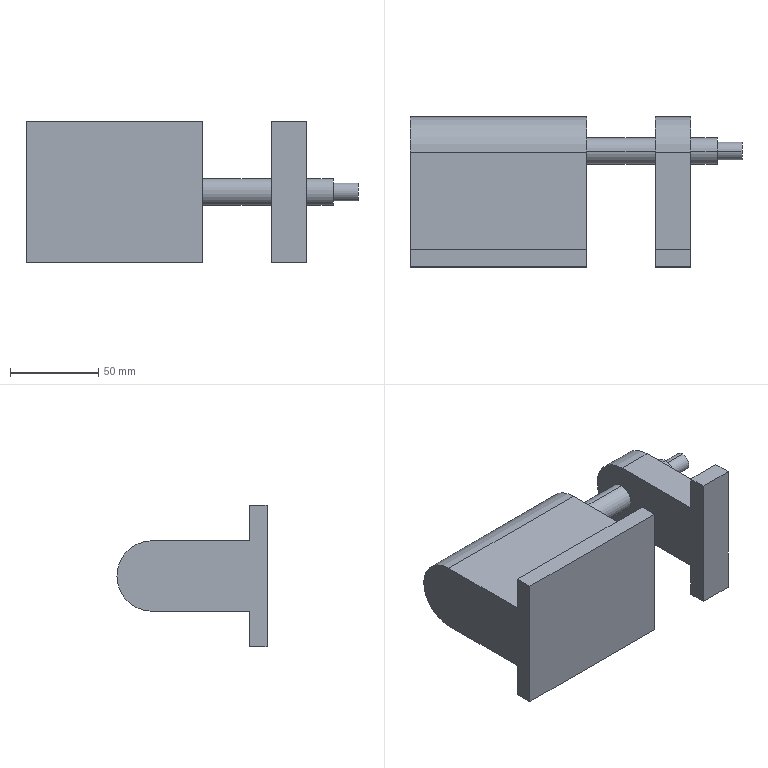Part | SolidWorks | features BaseBody 1 | 1 solid | 30 faces | box 188 x 85 x 80 mm | volume 446040 mm3 | plane 20 | cylinder 10 | commonest cylinder face diameters 15 x4 40 x4 10 x2
STEP:
#1=CARTESIAN_POINT('',(172.311,72.768,44.5));
#2=VERTEX_POINT('',#1);
#3=CARTESIAN_POINT('',(172.311,72.768,54.5));
#4=VERTEX_POINT('',#3);
#5=CARTESIAN_POINT('',(172.311,72.768,49.5));
#6=DIRECTION('',(1.,0.,0.));
#7=DIRECTION('',(0.,0.,-1.));
#8=AXIS2_PLACEMENT_3D('',#5,#6,#7);
#9=CIRCLE('',#8,5.);
#10=EDGE_CURVE('',#2,#4,#9,.T.);
#11=ORIENTED_EDGE('',*,*,#10,.F.);
#12=CARTESIAN_POINT('',(158.311,72.768,44.5));
#13=VERTEX_POINT('',#12);
#14=CARTESIAN_POINT('',(172.311,72.768,44.5));
#15=DIRECTION('',(-1.,0.,0.));
#16=VECTOR('',#15,1000.);
#17=LINE('',#14,#16);
#18=EDGE_CURVE('',#2,#13,#17,.T.);
#19=ORIENTED_EDGE('',*,*,#18,.T.);
#20=CARTESIAN_POINT('',(158.311,72.768,54.5));
#21=VERTEX_POINT('',#20);
#22=CARTESIAN_POINT('',(158.311,72.768,49.5));
#23=DIRECTION('',(1.,0.,0.));
#24=DIRECTION('',(0.,0.,-1.));
#25=AXIS2_PLACEMENT_3D('',#22,#23,#24);
#26=CIRCLE('',#25,5.);
#27=EDGE_CURVE('',#13,#21,#26,.T.);
#28=ORIENTED_EDGE('',*,*,#27,.T.);
#29=CARTESIAN_POINT('',(172.311,72.768,54.5));
#30=DIRECTION('',(-1.,0.,0.));
#31=VECTOR('',#30,1000.);
#32=LINE('',#29,#31);
#33=EDGE_CURVE('',#4,#21,#32,.T.);
#34=ORIENTED_EDGE('',*,*,#33,.F.);
#35=EDGE_LOOP('',(#11,#19,#28,#34));
#36=FACE_OUTER_BOUND('',#35,.T.);
#37=CARTESIAN_POINT('',(172.311,72.768,49.5));
#38=DIRECTION('',(-1.,0.,0.));
#39=DIRECTION('',(0.,0.,1.));
#40=AXIS2_PLACEMENT_3D('',#37,#38,#39);
#41=CYLINDRICAL_SURFACE('',#40,5.);
#42=ADVANCED_FACE('',(#36),#41,.T.);
#43=CARTESIAN_POINT('',(158.311,72.768,42.));
#44=VERTEX_POINT('',#43);
#45=CARTESIAN_POINT('',(158.311,72.768,57.));
#46=VERTEX_POINT('',#45);
#47=CARTESIAN_POINT('',(158.311,72.768,49.5));
#48=DIRECTION('',(1.,0.,0.));
#49=DIRECTION('',(0.,0.,-1.));
#50=AXIS2_PLACEMENT_3D('',#47,#48,#49);
#51=CIRCLE('',#50,7.5);
#52=EDGE_CURVE('',#44,#46,#51,.T.);
#53=ORIENTED_EDGE('',*,*,#52,.F.);
#54=CARTESIAN_POINT('',(143.218,72.768,42.));
#55=VERTEX_POINT('',#54);
#56=CARTESIAN_POINT('',(158.311,72.768,42.));
#57=DIRECTION('',(-1.,0.,0.));
#58=VECTOR('',#57,1000.);
#59=LINE('',#56,#58);
#60=EDGE_CURVE('',#44,#55,#59,.T.);
#61=ORIENTED_EDGE('',*,*,#60,.T.);
#62=CARTESIAN_POINT('',(143.218,72.768,57.));
#63=VERTEX_POINT('',#62);
#64=CARTESIAN_POINT('',(143.218,72.768,49.5));
#65=DIRECTION('',(1.,0.,0.));
#66=DIRECTION('',(0.,0.,-1.));
#67=AXIS2_PLACEMENT_3D('',#64,#65,#66);
#68=CIRCLE('',#67,7.5);
#69=EDGE_CURVE('',#55,#63,#68,.T.);
#70=ORIENTED_EDGE('',*,*,#69,.T.);
#71=CARTESIAN_POINT('',(158.311,72.768,57.));
#72=DIRECTION('',(-1.,0.,0.));
#73=VECTOR('',#72,1000.);
#74=LINE('',#71,#73);
#75=EDGE_CURVE('',#46,#63,#74,.T.);
#76=ORIENTED_EDGE('',*,*,#75,.F.);
#77=EDGE_LOOP('',(#53,#61,#70,#76));
#78=FACE_OUTER_BOUND('',#77,.T.);
#79=CARTESIAN_POINT('',(158.311,72.768,49.5));
#80=DIRECTION('',(-1.,0.,0.));
#81=DIRECTION('',(0.,0.,1.));
#82=AXIS2_PLACEMENT_3D('',#79,#80,#81);
#83=CYLINDRICAL_SURFACE('',#82,7.5);
#84=ADVANCED_FACE('',(#78),#83,.T.);
#85=CARTESIAN_POINT('',(123.218,72.768,57.));
#86=VERTEX_POINT('',#85);
#87=CARTESIAN_POINT('',(123.218,72.768,42.));
#88=VERTEX_POINT('',#87);
#89=CARTESIAN_POINT('',(123.218,72.768,49.5));
#90=DIRECTION('',(-1.,0.,0.));
#91=DIRECTION('',(0.,0.,-1.));
#92=AXIS2_PLACEMENT_3D('',#89,#90,#91);
#93=CIRCLE('',#92,7.5);
#94=EDGE_CURVE('',#86,#88,#93,.T.);
#95=ORIENTED_EDGE('',*,*,#94,.T.);
#96=CARTESIAN_POINT('',(84.311,72.768,42.));
#97=VERTEX_POINT('',#96);
#98=CARTESIAN_POINT('',(158.311,72.768,42.));
#99=DIRECTION('',(-1.,0.,0.));
#100=VECTOR('',#99,1000.);
#101=LINE('',#98,#100);
#102=EDGE_CURVE('',#88,#97,#101,.T.);
#103=ORIENTED_EDGE('',*,*,#102,.T.);
#104=CARTESIAN_POINT('',(84.311,72.768,57.));
#105=VERTEX_POINT('',#104);
#106=CARTESIAN_POINT('',(84.311,72.768,49.5));
#107=DIRECTION('',(1.,0.,0.));
#108=DIRECTION('',(0.,0.,1.));
#109=AXIS2_PLACEMENT_3D('',#106,#107,#108);
#110=CIRCLE('',#109,7.5);
#111=EDGE_CURVE('',#97,#105,#110,.T.);
#112=ORIENTED_EDGE('',*,*,#111,.T.);
#113=CARTESIAN_POINT('',(158.311,72.768,57.));
#114=DIRECTION('',(-1.,0.,0.));
#115=VECTOR('',#114,1000.);
#116=LINE('',#113,#115);
#117=EDGE_CURVE('',#86,#105,#116,.T.);
#118=ORIENTED_EDGE('',*,*,#117,.F.);
#119=EDGE_LOOP('',(#95,#103,#112,#118));
#120=FACE_OUTER_BOUND('',#119,.T.);
#121=CARTESIAN_POINT('',(158.311,72.768,49.5));
#122=DIRECTION('',(-1.,0.,0.));
#123=DIRECTION('',(0.,0.,1.));
#124=AXIS2_PLACEMENT_3D('',#121,#122,#123);
#125=CYLINDRICAL_SURFACE('',#124,7.5);
#126=ADVANCED_FACE('',(#120),#125,.T.);
#127=CARTESIAN_POINT('',(158.311,72.768,49.5));
#128=DIRECTION('',(1.,0.,0.));
#129=DIRECTION('',(0.,0.,-1.));
#130=AXIS2_PLACEMENT_3D('',#127,#128,#129);
#131=CIRCLE('',#130,7.5);
#132=EDGE_CURVE('',#46,#44,#131,.T.);
#133=ORIENTED_EDGE('',*,*,#132,.T.);
#134=ORIENTED_EDGE('',*,*,#52,.T.);
#135=EDGE_LOOP('',(#133,#134));
#136=FACE_OUTER_BOUND('',#135,.T.);
#137=CARTESIAN_POINT('',(158.311,72.768,49.5));
#138=DIRECTION('',(1.,0.,0.));
#139=DIRECTION('',(0.,0.,-1.));
#140=AXIS2_PLACEMENT_3D('',#137,#138,#139);
#141=CIRCLE('',#140,5.);
#142=EDGE_CURVE('',#21,#13,#141,.T.);
#143=ORIENTED_EDGE('',*,*,#142,.F.);
#144=ORIENTED_EDGE('',*,*,#27,.F.);
#145=EDGE_LOOP('',(#143,#144));
#146=FACE_BOUND('',#145,.T.);
#147=CARTESIAN_POINT('',(158.311,72.768,49.5));
#148=DIRECTION('',(1.,0.,0.));
#149=DIRECTION('',(0.,0.,-1.));
#150=AXIS2_PLACEMENT_3D('',#147,#148,#149);
#151=PLANE('',#150);
#152=ADVANCED_FACE('',(#136,#146),#151,.T.);
#153=CARTESIAN_POINT('',(84.311,72.138,29.5));
#154=VERTEX_POINT('',#153);
#155=CARTESIAN_POINT('',(84.311,17.138,29.5));
#156=VERTEX_POINT('',#155);
#157=CARTESIAN_POINT('',(84.311,92.138,29.5));
#158=DIRECTION('',(0.,-1.,0.));
#159=VECTOR('',#158,1000.);
#160=LINE('',#157,#159);
#161=EDGE_CURVE('',#154,#156,#160,.T.);
#162=ORIENTED_EDGE('',*,*,#161,.F.);
#163=CARTESIAN_POINT('',(84.311,92.138,49.5));
#164=VERTEX_POINT('',#163);
#165=CARTESIAN_POINT('',(84.311,72.138,49.5));
#166=DIRECTION('',(1.,0.,0.));
#167=DIRECTION('',(0.,0.,1.));
#168=AXIS2_PLACEMENT_3D('',#165,#166,#167);
#169=CIRCLE('',#168,20.);
#170=EDGE_CURVE('',#154,#164,#169,.T.);
#171=ORIENTED_EDGE('',*,*,#170,.T.);
#172=CARTESIAN_POINT('',(84.311,72.138,69.5));
#173=VERTEX_POINT('',#172);
#174=CARTESIAN_POINT('',(84.311,72.138,49.5));
#175=DIRECTION('',(1.,0.,0.));
#176=DIRECTION('',(0.,0.,1.));
#177=AXIS2_PLACEMENT_3D('',#174,#175,#176);
#178=CIRCLE('',#177,20.);
#179=EDGE_CURVE('',#164,#173,#178,.T.);
#180=ORIENTED_EDGE('',*,*,#179,.T.);
#181=CARTESIAN_POINT('',(84.311,17.138,69.5));
#182=VERTEX_POINT('',#181);
#183=CARTESIAN_POINT('',(84.311,92.138,69.5));
#184=DIRECTION('',(0.,-1.,0.));
#185=VECTOR('',#184,1000.);
#186=LINE('',#183,#185);
#187=EDGE_CURVE('',#173,#182,#186,.T.);
#188=ORIENTED_EDGE('',*,*,#187,.T.);
#189=CARTESIAN_POINT('',(84.311,17.138,89.5));
#190=VERTEX_POINT('',#189);
#191=CARTESIAN_POINT('',(84.311,17.138,89.5));
#192=DIRECTION('',(0.,0.,-1.));
#193=VECTOR('',#192,1000.);
#194=LINE('',#191,#193);
#195=EDGE_CURVE('',#190,#182,#194,.T.);
#196=ORIENTED_EDGE('',*,*,#195,.F.);
#197=CARTESIAN_POINT('',(84.311,7.138,89.5));
#198=VERTEX_POINT('',#197);
#199=CARTESIAN_POINT('',(84.311,17.138,89.5));
#200=DIRECTION('',(0.,-1.,0.));
#201=VECTOR('',#200,1000.);
#202=LINE('',#199,#201);
#203=EDGE_CURVE('',#190,#198,#202,.T.);
#204=ORIENTED_EDGE('',*,*,#203,.T.);
#205=CARTESIAN_POINT('',(84.311,7.138,9.5));
#206=VERTEX_POINT('',#205);
#207=CARTESIAN_POINT('',(84.311,7.138,89.5));
#208=DIRECTION('',(0.,0.,-1.));
#209=VECTOR('',#208,1000.);
#210=LINE('',#207,#209);
#211=EDGE_CURVE('',#198,#206,#210,.T.);
#212=ORIENTED_EDGE('',*,*,#211,.T.);
#213=CARTESIAN_POINT('',(84.311,17.138,9.5));
#214=VERTEX_POINT('',#213);
#215=CARTESIAN_POINT('',(84.311,17.138,9.5));
#216=DIRECTION('',(0.,-1.,0.));
#217=VECTOR('',#216,1000.);
#218=LINE('',#215,#217);
#219=EDGE_CURVE('',#214,#206,#218,.T.);
#220=ORIENTED_EDGE('',*,*,#219,.F.);
#221=CARTESIAN_POINT('',(84.311,17.138,89.5));
#222=DIRECTION('',(0.,0.,-1.));
#223=VECTOR('',#222,1000.);
#224=LINE('',#221,#223);
#225=EDGE_CURVE('',#156,#214,#224,.T.);
#226=ORIENTED_EDGE('',*,*,#225,.F.);
#227=EDGE_LOOP('',(#162,#171,#180,#188,#196,#204,#212,#220,#226));
#228=FACE_OUTER_BOUND('',#227,.T.);
#229=CARTESIAN_POINT('',(84.311,72.768,49.5));
#230=DIRECTION('',(1.,0.,0.));
#231=DIRECTION('',(0.,0.,1.));
#232=AXIS2_PLACEMENT_3D('',#229,#230,#231);
#233=CIRCLE('',#232,7.5);
#234=EDGE_CURVE('',#105,#97,#233,.T.);
#235=ORIENTED_EDGE('',*,*,#234,.F.);
#236=ORIENTED_EDGE('',*,*,#111,.F.);
#237=EDGE_LOOP('',(#235,#236));
#238=FACE_BOUND('',#237,.T.);
#239=CARTESIAN_POINT('',(84.311,17.138,89.5));
#240=DIRECTION('',(-1.,0.,0.));
#241=DIRECTION('',(0.,0.,1.));
#242=AXIS2_PLACEMENT_3D('',#239,#240,#241);
#243=PLANE('',#242);
#244=ADVANCED_FACE('',(#228,#238),#243,.F.);
#245=CARTESIAN_POINT('',(-15.689,17.138,69.5));
#246=VERTEX_POINT('',#245);
#247=CARTESIAN_POINT('',(84.311,17.138,69.5));
#248=DIRECTION('',(1.,0.,0.));
#249=VECTOR('',#248,1000.);
#250=LINE('',#247,#249);
#251=EDGE_CURVE('',#246,#182,#250,.T.);
#252=ORIENTED_EDGE('',*,*,#251,.F.);
#253=CARTESIAN_POINT('',(-15.689,17.138,89.5));
#254=VERTEX_POINT('',#253);
#255=CARTESIAN_POINT('',(-15.689,17.138,9.5));
#256=DIRECTION('',(0.,0.,1.));
#257=VECTOR('',#256,1000.);
#258=LINE('',#255,#257);
#259=EDGE_CURVE('',#246,#254,#258,.T.);
#260=ORIENTED_EDGE('',*,*,#259,.T.);
#261=CARTESIAN_POINT('',(-15.689,17.138,89.5));
#262=DIRECTION('',(1.,0.,0.));
#263=VECTOR('',#262,1000.);
#264=LINE('',#261,#263);
#265=EDGE_CURVE('',#254,#190,#264,.T.);
#266=ORIENTED_EDGE('',*,*,#265,.T.);
#267=ORIENTED_EDGE('',*,*,#195,.T.);
#268=EDGE_LOOP('',(#252,#260,#266,#267));
#269=FACE_OUTER_BOUND('',#268,.T.);
#270=CARTESIAN_POINT('',(-546.782,17.138,0.));
#271=DIRECTION('',(0.,1.,0.));
#272=DIRECTION('',(0.,0.,1.));
#273=AXIS2_PLACEMENT_3D('',#270,#271,#272);
#274=PLANE('',#273);
#275=ADVANCED_FACE('',(#269),#274,.T.);
#276=CARTESIAN_POINT('',(123.218,17.138,69.5));
#277=VERTEX_POINT('',#276);
#278=CARTESIAN_POINT('',(143.218,17.138,69.5));
#279=VERTEX_POINT('',#278);
#280=CARTESIAN_POINT('',(123.218,17.138,69.5));
#281=DIRECTION('',(1.,0.,0.));
#282=VECTOR('',#281,1000.);
#283=LINE('',#280,#282);
#284=EDGE_CURVE('',#277,#279,#283,.T.);
#285=ORIENTED_EDGE('',*,*,#284,.F.);
#286=CARTESIAN_POINT('',(123.218,17.138,89.5));
#287=VERTEX_POINT('',#286);
#288=CARTESIAN_POINT('',(123.218,17.138,15.727));
#289=DIRECTION('',(0.,0.,1.));
#290=VECTOR('',#289,1000.);
#291=LINE('',#288,#290);
#292=EDGE_CURVE('',#277,#287,#291,.T.);
#293=ORIENTED_EDGE('',*,*,#292,.T.);
#294=CARTESIAN_POINT('',(143.218,17.138,89.5));
#295=VERTEX_POINT('',#294);
#296=CARTESIAN_POINT('',(123.218,17.138,89.5));
#297=DIRECTION('',(1.,0.,0.));
#298=VECTOR('',#297,1000.);
#299=LINE('',#296,#298);
#300=EDGE_CURVE('',#287,#295,#299,.T.);
#301=ORIENTED_EDGE('',*,*,#300,.T.);
#302=CARTESIAN_POINT('',(143.218,17.138,15.727));
#303=DIRECTION('',(0.,0.,-1.));
#304=VECTOR('',#303,1000.);
#305=LINE('',#302,#304);
#306=EDGE_CURVE('',#295,#279,#305,.T.);
#307=ORIENTED_EDGE('',*,*,#306,.T.);
#308=EDGE_LOOP('',(#285,#293,#301,#307));
#309=FACE_OUTER_BOUND('',#308,.T.);
#310=CARTESIAN_POINT('',(-546.782,17.138,0.));
#311=DIRECTION('',(0.,-1.,0.));
#312=DIRECTION('',(0.,0.,-1.));
#313=AXIS2_PLACEMENT_3D('',#310,#311,#312);
#314=PLANE('',#313);
#315=ADVANCED_FACE('',(#309),#314,.F.);
#316=CARTESIAN_POINT('',(143.218,17.138,29.5));
#317=VERTEX_POINT('',#316);
#318=CARTESIAN_POINT('',(123.218,17.138,29.5));
#319=VERTEX_POINT('',#318);
#320=CARTESIAN_POINT('',(123.218,17.138,29.5));
#321=DIRECTION('',(-1.,0.,0.));
#322=VECTOR('',#321,1000.);
#323=LINE('',#320,#322);
#324=EDGE_CURVE('',#317,#319,#323,.T.);
#325=ORIENTED_EDGE('',*,*,#324,.F.);
#326=CARTESIAN_POINT('',(143.218,17.138,9.5));
#327=VERTEX_POINT('',#326);
#328=CARTESIAN_POINT('',(143.218,17.138,15.727));
#329=DIRECTION('',(0.,0.,-1.));
#330=VECTOR('',#329,1000.);
#331=LINE('',#328,#330);
#332=EDGE_CURVE('',#317,#327,#331,.T.);
#333=ORIENTED_EDGE('',*,*,#332,.T.);
#334=CARTESIAN_POINT('',(123.218,17.138,9.5));
#335=VERTEX_POINT('',#334);
#336=CARTESIAN_POINT('',(123.218,17.138,9.5));
#337=DIRECTION('',(-1.,0.,0.));
#338=VECTOR('',#337,1000.);
#339=LINE('',#336,#338);
#340=EDGE_CURVE('',#327,#335,#339,.T.);
#341=ORIENTED_EDGE('',*,*,#340,.T.);
#342=CARTESIAN_POINT('',(123.218,17.138,15.727));
#343=DIRECTION('',(0.,0.,1.));
#344=VECTOR('',#343,1000.);
#345=LINE('',#342,#344);
#346=EDGE_CURVE('',#335,#319,#345,.T.);
#347=ORIENTED_EDGE('',*,*,#346,.T.);
#348=EDGE_LOOP('',(#325,#333,#341,#347));
#349=FACE_OUTER_BOUND('',#348,.T.);
#350=CARTESIAN_POINT('',(-546.782,17.138,0.));
#351=DIRECTION('',(0.,-1.,0.));
#352=DIRECTION('',(0.,0.,-1.));
#353=AXIS2_PLACEMENT_3D('',#350,#351,#352);
#354=PLANE('',#353);
#355=ADVANCED_FACE('',(#349),#354,.F.);
#356=CARTESIAN_POINT('',(143.218,7.138,9.5));
#357=VERTEX_POINT('',#356);
#358=CARTESIAN_POINT('',(123.218,7.138,9.5));
#359=VERTEX_POINT('',#358);
#360=CARTESIAN_POINT('',(123.218,7.138,9.5));
#361=DIRECTION('',(-1.,0.,0.));
#362=VECTOR('',#361,1000.);
#363=LINE('',#360,#362);
#364=EDGE_CURVE('',#357,#359,#363,.T.);
#365=ORIENTED_EDGE('',*,*,#364,.T.);
#366=CARTESIAN_POINT('',(123.218,17.138,9.5));
#367=DIRECTION('',(0.,-1.,0.));
#368=VECTOR('',#367,1000.);
#369=LINE('',#366,#368);
#370=EDGE_CURVE('',#335,#359,#369,.T.);
#371=ORIENTED_EDGE('',*,*,#370,.F.);
#372=ORIENTED_EDGE('',*,*,#340,.F.);
#373=CARTESIAN_POINT('',(143.218,17.138,9.5));
#374=DIRECTION('',(0.,-1.,0.));
#375=VECTOR('',#374,1000.);
#376=LINE('',#373,#375);
#377=EDGE_CURVE('',#327,#357,#376,.T.);
#378=ORIENTED_EDGE('',*,*,#377,.T.);
#379=EDGE_LOOP('',(#365,#371,#372,#378));
#380=FACE_OUTER_BOUND('',#379,.T.);
#381=CARTESIAN_POINT('',(123.218,17.138,9.5));
#382=DIRECTION('',(0.,0.,1.));
#383=DIRECTION('',(1.,0.,0.));
#384=AXIS2_PLACEMENT_3D('',#381,#382,#383);
#385=PLANE('',#384);
#386=ADVANCED_FACE('',(#380),#385,.F.);
#387=ORIENTED_EDGE('',*,*,#94,.F.);
#388=CARTESIAN_POINT('',(123.218,72.768,49.5));
#389=DIRECTION('',(-1.,0.,0.));
#390=DIRECTION('',(0.,0.,-1.));
#391=AXIS2_PLACEMENT_3D('',#388,#389,#390);
#392=CIRCLE('',#391,7.5);
#393=EDGE_CURVE('',#88,#86,#392,.T.);
#394=ORIENTED_EDGE('',*,*,#393,.F.);
#395=EDGE_LOOP('',(#387,#394));
#396=FACE_BOUND('',#395,.T.);
#397=CARTESIAN_POINT('',(123.218,72.138,69.5));
#398=VERTEX_POINT('',#397);
#399=CARTESIAN_POINT('',(123.218,92.138,49.5));
#400=VERTEX_POINT('',#399);
#401=CARTESIAN_POINT('',(123.218,72.138,49.5));
#402=DIRECTION('',(-1.,0.,0.));
#403=DIRECTION('',(0.,0.,-1.));
#404=AXIS2_PLACEMENT_3D('',#401,#402,#403);
#405=CIRCLE('',#404,20.);
#406=EDGE_CURVE('',#398,#400,#405,.T.);
#407=ORIENTED_EDGE('',*,*,#406,.T.);
#408=CARTESIAN_POINT('',(123.218,72.138,29.5));
#409=VERTEX_POINT('',#408);
#410=CARTESIAN_POINT('',(123.218,72.138,49.5));
#411=DIRECTION('',(-1.,0.,0.));
#412=DIRECTION('',(0.,0.,-1.));
#413=AXIS2_PLACEMENT_3D('',#410,#411,#412);
#414=CIRCLE('',#413,20.);
#415=EDGE_CURVE('',#400,#409,#414,.T.);
#416=ORIENTED_EDGE('',*,*,#415,.T.);
#417=CARTESIAN_POINT('',(123.218,92.138,29.5));
#418=DIRECTION('',(0.,-1.,0.));
#419=VECTOR('',#418,1000.);
#420=LINE('',#417,#419);
#421=EDGE_CURVE('',#409,#319,#420,.T.);
#422=ORIENTED_EDGE('',*,*,#421,.T.);
#423=ORIENTED_EDGE('',*,*,#346,.F.);
#424=ORIENTED_EDGE('',*,*,#370,.T.);
#425=CARTESIAN_POINT('',(123.218,7.138,89.5));
#426=VERTEX_POINT('',#425);
#427=CARTESIAN_POINT('',(123.218,7.138,15.727));
#428=DIRECTION('',(0.,0.,1.));
#429=VECTOR('',#428,1000.);
#430=LINE('',#427,#429);
#431=EDGE_CURVE('',#359,#426,#430,.T.);
#432=ORIENTED_EDGE('',*,*,#431,.T.);
#433=CARTESIAN_POINT('',(123.218,17.138,89.5));
#434=DIRECTION('',(0.,-1.,0.));
#435=VECTOR('',#434,1000.);
#436=LINE('',#433,#435);
#437=EDGE_CURVE('',#287,#426,#436,.T.);
#438=ORIENTED_EDGE('',*,*,#437,.F.);
#439=ORIENTED_EDGE('',*,*,#292,.F.);
#440=CARTESIAN_POINT('',(123.218,92.138,69.5));
#441=DIRECTION('',(0.,-1.,0.));
#442=VECTOR('',#441,1000.);
#443=LINE('',#440,#442);
#444=EDGE_CURVE('',#398,#277,#443,.T.);
#445=ORIENTED_EDGE('',*,*,#444,.F.);
#446=EDGE_LOOP('',(#407,#416,#422,#423,#424,#432,#438,#439,#445));
#447=FACE_OUTER_BOUND('',#446,.T.);
#448=CARTESIAN_POINT('',(123.218,17.138,15.727));
#449=DIRECTION('',(1.,0.,0.));
#450=DIRECTION('',(0.,0.,-1.));
#451=AXIS2_PLACEMENT_3D('',#448,#449,#450);
#452=PLANE('',#451);
#453=ADVANCED_FACE('',(#396,#447),#452,.F.);
#454=CARTESIAN_POINT('',(143.218,7.138,89.5));
#455=VERTEX_POINT('',#454);
#456=CARTESIAN_POINT('',(123.218,7.138,89.5));
#457=DIRECTION('',(1.,0.,0.));
#458=VECTOR('',#457,1000.);
#459=LINE('',#456,#458);
#460=EDGE_CURVE('',#426,#455,#459,.T.);
#461=ORIENTED_EDGE('',*,*,#460,.T.);
#462=CARTESIAN_POINT('',(143.218,17.138,89.5));
#463=DIRECTION('',(0.,-1.,0.));
#464=VECTOR('',#463,1000.);
#465=LINE('',#462,#464);
#466=EDGE_CURVE('',#295,#455,#465,.T.);
#467=ORIENTED_EDGE('',*,*,#466,.F.);
#468=ORIENTED_EDGE('',*,*,#300,.F.);
#469=ORIENTED_EDGE('',*,*,#437,.T.);
#470=EDGE_LOOP('',(#461,#467,#468,#469));
#471=FACE_OUTER_BOUND('',#470,.T.);
#472=CARTESIAN_POINT('',(123.218,17.138,89.5));
#473=DIRECTION('',(0.,0.,-1.));
#474=DIRECTION('',(-1.,0.,0.));
#475=AXIS2_PLACEMENT_3D('',#472,#473,#474);
#476=PLANE('',#475);
#477=ADVANCED_FACE('',(#471),#476,.F.);
#478=CARTESIAN_POINT('',(143.218,72.768,49.5));
#479=DIRECTION('',(1.,0.,0.));
#480=DIRECTION('',(0.,0.,-1.));
#481=AXIS2_PLACEMENT_3D('',#478,#479,#480);
#482=CIRCLE('',#481,7.5);
#483=EDGE_CURVE('',#63,#55,#482,.T.);
#484=ORIENTED_EDGE('',*,*,#483,.F.);
#485=ORIENTED_EDGE('',*,*,#69,.F.);
#486=EDGE_LOOP('',(#484,#485));
#487=FACE_BOUND('',#486,.T.);
#488=CARTESIAN_POINT('',(143.218,72.138,29.5));
#489=VERTEX_POINT('',#488);
#490=CARTESIAN_POINT('',(143.218,92.138,29.5));
#491=DIRECTION('',(0.,-1.,0.));
#492=VECTOR('',#491,1000.);
#493=LINE('',#490,#492);
#494=EDGE_CURVE('',#489,#317,#493,.T.);
#495=ORIENTED_EDGE('',*,*,#494,.F.);
#496=CARTESIAN_POINT('',(143.218,92.138,49.5));
#497=VERTEX_POINT('',#496);
#498=CARTESIAN_POINT('',(143.218,72.138,49.5));
#499=DIRECTION('',(1.,0.,0.));
#500=DIRECTION('',(0.,0.,1.));
#501=AXIS2_PLACEMENT_3D('',#498,#499,#500);
#502=CIRCLE('',#501,20.);
#503=EDGE_CURVE('',#489,#497,#502,.T.);
#504=ORIENTED_EDGE('',*,*,#503,.T.);
#505=CARTESIAN_POINT('',(143.218,72.138,69.5));
#506=VERTEX_POINT('',#505);
#507=CARTESIAN_POINT('',(143.218,72.138,49.5));
#508=DIRECTION('',(1.,0.,0.));
#509=DIRECTION('',(0.,0.,1.));
#510=AXIS2_PLACEMENT_3D('',#507,#508,#509);
#511=CIRCLE('',#510,20.);
#512=EDGE_CURVE('',#497,#506,#511,.T.);
#513=ORIENTED_EDGE('',*,*,#512,.T.);
#514=CARTESIAN_POINT('',(143.218,92.138,69.5));
#515=DIRECTION('',(0.,-1.,0.));
#516=VECTOR('',#515,1000.);
#517=LINE('',#514,#516);
#518=EDGE_CURVE('',#506,#279,#517,.T.);
#519=ORIENTED_EDGE('',*,*,#518,.T.);
#520=ORIENTED_EDGE('',*,*,#306,.F.);
#521=ORIENTED_EDGE('',*,*,#466,.T.);
#522=CARTESIAN_POINT('',(143.218,7.138,15.727));
#523=DIRECTION('',(0.,0.,-1.));
#524=VECTOR('',#523,1000.);
#525=LINE('',#522,#524);
#526=EDGE_CURVE('',#455,#357,#525,.T.);
#527=ORIENTED_EDGE('',*,*,#526,.T.);
#528=ORIENTED_EDGE('',*,*,#377,.F.);
#529=ORIENTED_EDGE('',*,*,#332,.F.);
#530=EDGE_LOOP('',(#495,#504,#513,#519,#520,#521,#527,#528,#529));
#531=FACE_OUTER_BOUND('',#530,.T.);
#532=CARTESIAN_POINT('',(143.218,17.138,15.727));
#533=DIRECTION('',(-1.,0.,0.));
#534=DIRECTION('',(0.,0.,1.));
#535=AXIS2_PLACEMENT_3D('',#532,#533,#534);
#536=PLANE('',#535);
#537=ADVANCED_FACE('',(#487,#531),#536,.F.);
#538=ORIENTED_EDGE('',*,*,#518,.F.);
#539=CARTESIAN_POINT('',(123.218,72.138,69.5));
#540=DIRECTION('',(-1.,0.,0.));
#541=VECTOR('',#540,1000.);
#542=LINE('',#539,#541);
#543=EDGE_CURVE('',#506,#398,#542,.T.);
#544=ORIENTED_EDGE('',*,*,#543,.T.);
#545=ORIENTED_EDGE('',*,*,#444,.T.);
#546=ORIENTED_EDGE('',*,*,#284,.T.);
#547=EDGE_LOOP('',(#538,#544,#545,#546));
#548=FACE_OUTER_BOUND('',#547,.T.);
#549=CARTESIAN_POINT('',(123.218,92.138,69.5));
#550=DIRECTION('',(0.,0.,-1.));
#551=DIRECTION('',(-1.,0.,0.));
#552=AXIS2_PLACEMENT_3D('',#549,#550,#551);
#553=PLANE('',#552);
#554=ADVANCED_FACE('',(#548),#553,.F.);
#555=ORIENTED_EDGE('',*,*,#421,.F.);
#556=CARTESIAN_POINT('',(143.218,72.138,29.5));
#557=DIRECTION('',(1.,0.,0.));
#558=VECTOR('',#557,1000.);
#559=LINE('',#556,#558);
#560=EDGE_CURVE('',#409,#489,#559,.T.);
#561=ORIENTED_EDGE('',*,*,#560,.T.);
#562=ORIENTED_EDGE('',*,*,#494,.T.);
#563=ORIENTED_EDGE('',*,*,#324,.T.);
#564=EDGE_LOOP('',(#555,#561,#562,#563));
#565=FACE_OUTER_BOUND('',#564,.T.);
#566=CARTESIAN_POINT('',(123.218,92.138,29.5));
#567=DIRECTION('',(0.,0.,1.));
#568=DIRECTION('',(1.,0.,0.));
#569=AXIS2_PLACEMENT_3D('',#566,#567,#568);
#570=PLANE('',#569);
#571=ADVANCED_FACE('',(#565),#570,.F.);
#572=ORIENTED_EDGE('',*,*,#543,.F.);
#573=ORIENTED_EDGE('',*,*,#512,.F.);
#574=CARTESIAN_POINT('',(143.218,92.138,49.5));
#575=DIRECTION('',(1.,0.,0.));
#576=VECTOR('',#575,1000.);
#577=LINE('',#574,#576);
#578=EDGE_CURVE('',#400,#497,#577,.T.);
#579=ORIENTED_EDGE('',*,*,#578,.F.);
#580=ORIENTED_EDGE('',*,*,#406,.F.);
#581=EDGE_LOOP('',(#572,#573,#579,#580));
#582=FACE_OUTER_BOUND('',#581,.T.);
#583=CARTESIAN_POINT('',(-546.782,72.138,49.5));
#584=DIRECTION('',(-1.,0.,0.));
#585=DIRECTION('',(0.,0.,1.));
#586=AXIS2_PLACEMENT_3D('',#583,#584,#585);
#587=CYLINDRICAL_SURFACE('',#586,20.);
#588=ADVANCED_FACE('',(#582),#587,.T.);
#589=ORIENTED_EDGE('',*,*,#503,.F.);
#590=ORIENTED_EDGE('',*,*,#560,.F.);
#591=ORIENTED_EDGE('',*,*,#415,.F.);
#592=ORIENTED_EDGE('',*,*,#578,.T.);
#593=EDGE_LOOP('',(#589,#590,#591,#592));
#594=FACE_OUTER_BOUND('',#593,.T.);
#595=CARTESIAN_POINT('',(-546.782,72.138,49.5));
#596=DIRECTION('',(1.,0.,0.));
#597=DIRECTION('',(0.,0.,-1.));
#598=AXIS2_PLACEMENT_3D('',#595,#596,#597);
#599=CYLINDRICAL_SURFACE('',#598,20.);
#600=ADVANCED_FACE('',(#594),#599,.T.);
#601=CARTESIAN_POINT('',(-15.689,7.138,9.5));
#602=VERTEX_POINT('',#601);
#603=CARTESIAN_POINT('',(84.311,7.138,9.5));
#604=DIRECTION('',(-1.,0.,0.));
#605=VECTOR('',#604,1000.);
#606=LINE('',#603,#605);
#607=EDGE_CURVE('',#206,#602,#606,.T.);
#608=ORIENTED_EDGE('',*,*,#607,.T.);
#609=CARTESIAN_POINT('',(-15.689,17.138,9.5));
#610=VERTEX_POINT('',#609);
#611=CARTESIAN_POINT('',(-15.689,17.138,9.5));
#612=DIRECTION('',(0.,-1.,0.));
#613=VECTOR('',#612,1000.);
#614=LINE('',#611,#613);
#615=EDGE_CURVE('',#610,#602,#614,.T.);
#616=ORIENTED_EDGE('',*,*,#615,.F.);
#617=CARTESIAN_POINT('',(84.311,17.138,9.5));
#618=DIRECTION('',(-1.,0.,0.));
#619=VECTOR('',#618,1000.);
#620=LINE('',#617,#619);
#621=EDGE_CURVE('',#214,#610,#620,.T.);
#622=ORIENTED_EDGE('',*,*,#621,.F.);
#623=ORIENTED_EDGE('',*,*,#219,.T.);
#624=EDGE_LOOP('',(#608,#616,#622,#623));
#625=FACE_OUTER_BOUND('',#624,.T.);
#626=CARTESIAN_POINT('',(84.311,17.138,9.5));
#627=DIRECTION('',(0.,0.,1.));
#628=DIRECTION('',(1.,0.,0.));
#629=AXIS2_PLACEMENT_3D('',#626,#627,#628);
#630=PLANE('',#629);
#631=ADVANCED_FACE('',(#625),#630,.F.);
#632=CARTESIAN_POINT('',(-15.689,72.138,69.5));
#633=VERTEX_POINT('',#632);
#634=CARTESIAN_POINT('',(-15.689,92.138,49.5));
#635=VERTEX_POINT('',#634);
#636=CARTESIAN_POINT('',(-15.689,72.138,49.5));
#637=DIRECTION('',(-1.,0.,0.));
#638=DIRECTION('',(0.,0.,-1.));
#639=AXIS2_PLACEMENT_3D('',#636,#637,#638);
#640=CIRCLE('',#639,20.);
#641=EDGE_CURVE('',#633,#635,#640,.T.);
#642=ORIENTED_EDGE('',*,*,#641,.T.);
#643=CARTESIAN_POINT('',(-15.689,72.138,29.5));
#644=VERTEX_POINT('',#643);
#645=CARTESIAN_POINT('',(-15.689,72.138,49.5));
#646=DIRECTION('',(-1.,0.,0.));
#647=DIRECTION('',(0.,0.,-1.));
#648=AXIS2_PLACEMENT_3D('',#645,#646,#647);
#649=CIRCLE('',#648,20.);
#650=EDGE_CURVE('',#635,#644,#649,.T.);
#651=ORIENTED_EDGE('',*,*,#650,.T.);
#652=CARTESIAN_POINT('',(-15.689,17.138,29.5));
#653=VERTEX_POINT('',#652);
#654=CARTESIAN_POINT('',(-15.689,92.138,29.5));
#655=DIRECTION('',(0.,-1.,0.));
#656=VECTOR('',#655,1000.);
#657=LINE('',#654,#656);
#658=EDGE_CURVE('',#644,#653,#657,.T.);
#659=ORIENTED_EDGE('',*,*,#658,.T.);
#660=CARTESIAN_POINT('',(-15.689,17.138,9.5));
#661=DIRECTION('',(0.,0.,1.));
#662=VECTOR('',#661,1000.);
#663=LINE('',#660,#662);
#664=EDGE_CURVE('',#610,#653,#663,.T.);
#665=ORIENTED_EDGE('',*,*,#664,.F.);
#666=ORIENTED_EDGE('',*,*,#615,.T.);
#667=CARTESIAN_POINT('',(-15.689,7.138,89.5));
#668=VERTEX_POINT('',#667);
#669=CARTESIAN_POINT('',(-15.689,7.138,9.5));
#670=DIRECTION('',(0.,0.,1.));
#671=VECTOR('',#670,1000.);
#672=LINE('',#669,#671);
#673=EDGE_CURVE('',#602,#668,#672,.T.);
#674=ORIENTED_EDGE('',*,*,#673,.T.);
#675=CARTESIAN_POINT('',(-15.689,17.138,89.5));
#676=DIRECTION('',(0.,-1.,0.));
#677=VECTOR('',#676,1000.);
#678=LINE('',#675,#677);
#679=EDGE_CURVE('',#254,#668,#678,.T.);
#680=ORIENTED_EDGE('',*,*,#679,.F.);
#681=ORIENTED_EDGE('',*,*,#259,.F.);
#682=CARTESIAN_POINT('',(-15.689,92.138,69.5));
#683=DIRECTION('',(0.,-1.,0.));
#684=VECTOR('',#683,1000.);
#685=LINE('',#682,#684);
#686=EDGE_CURVE('',#633,#246,#685,.T.);
#687=ORIENTED_EDGE('',*,*,#686,.F.);
#688=EDGE_LOOP('',(#642,#651,#659,#665,#666,#674,#680,#681,#687));
#689=FACE_OUTER_BOUND('',#688,.T.);
#690=CARTESIAN_POINT('',(-15.689,17.138,9.5));
#691=DIRECTION('',(1.,0.,0.));
#692=DIRECTION('',(0.,0.,-1.));
#693=AXIS2_PLACEMENT_3D('',#690,#691,#692);
#694=PLANE('',#693);
#695=ADVANCED_FACE('',(#689),#694,.F.);
#696=CARTESIAN_POINT('',(-15.689,7.138,89.5));
#697=DIRECTION('',(1.,0.,0.));
#698=VECTOR('',#697,1000.);
#699=LINE('',#696,#698);
#700=EDGE_CURVE('',#668,#198,#699,.T.);
#701=ORIENTED_EDGE('',*,*,#700,.T.);
#702=ORIENTED_EDGE('',*,*,#203,.F.);
#703=ORIENTED_EDGE('',*,*,#265,.F.);
#704=ORIENTED_EDGE('',*,*,#679,.T.);
#705=EDGE_LOOP('',(#701,#702,#703,#704));
#706=FACE_OUTER_BOUND('',#705,.T.);
#707=CARTESIAN_POINT('',(-15.689,17.138,89.5));
#708=DIRECTION('',(0.,0.,-1.));
#709=DIRECTION('',(-1.,0.,0.));
#710=AXIS2_PLACEMENT_3D('',#707,#708,#709);
#711=PLANE('',#710);
#712=ADVANCED_FACE('',(#706),#711,.F.);
#713=CARTESIAN_POINT('',(84.311,17.138,29.5));
#714=DIRECTION('',(-1.,0.,0.));
#715=VECTOR('',#714,1000.);
#716=LINE('',#713,#715);
#717=EDGE_CURVE('',#156,#653,#716,.T.);
#718=ORIENTED_EDGE('',*,*,#717,.F.);
#719=ORIENTED_EDGE('',*,*,#225,.T.);
#720=ORIENTED_EDGE('',*,*,#621,.T.);
#721=ORIENTED_EDGE('',*,*,#664,.T.);
#722=EDGE_LOOP('',(#718,#719,#720,#721));
#723=FACE_OUTER_BOUND('',#722,.T.);
#724=CARTESIAN_POINT('',(-546.782,17.138,0.));
#725=DIRECTION('',(0.,1.,0.));
#726=DIRECTION('',(0.,0.,1.));
#727=AXIS2_PLACEMENT_3D('',#724,#725,#726);
#728=PLANE('',#727);
#729=ADVANCED_FACE('',(#723),#728,.T.);
#730=ORIENTED_EDGE('',*,*,#658,.F.);
#731=CARTESIAN_POINT('',(84.311,72.138,29.5));
#732=DIRECTION('',(1.,0.,0.));
#733=VECTOR('',#732,1000.);
#734=LINE('',#731,#733);
#735=EDGE_CURVE('',#644,#154,#734,.T.);
#736=ORIENTED_EDGE('',*,*,#735,.T.);
#737=ORIENTED_EDGE('',*,*,#161,.T.);
#738=ORIENTED_EDGE('',*,*,#717,.T.);
#739=EDGE_LOOP('',(#730,#736,#737,#738));
#740=FACE_OUTER_BOUND('',#739,.T.);
#741=CARTESIAN_POINT('',(84.311,92.138,29.5));
#742=DIRECTION('',(0.,0.,1.));
#743=DIRECTION('',(1.,0.,0.));
#744=AXIS2_PLACEMENT_3D('',#741,#742,#743);
#745=PLANE('',#744);
#746=ADVANCED_FACE('',(#740),#745,.F.);
#747=ORIENTED_EDGE('',*,*,#187,.F.);
#748=CARTESIAN_POINT('',(84.311,72.138,69.5));
#749=DIRECTION('',(-1.,0.,0.));
#750=VECTOR('',#749,1000.);
#751=LINE('',#748,#750);
#752=EDGE_CURVE('',#173,#633,#751,.T.);
#753=ORIENTED_EDGE('',*,*,#752,.T.);
#754=ORIENTED_EDGE('',*,*,#686,.T.);
#755=ORIENTED_EDGE('',*,*,#251,.T.);
#756=EDGE_LOOP('',(#747,#753,#754,#755));
#757=FACE_OUTER_BOUND('',#756,.T.);
#758=CARTESIAN_POINT('',(84.311,92.138,69.5));
#759=DIRECTION('',(0.,0.,-1.));
#760=DIRECTION('',(-1.,0.,0.));
#761=AXIS2_PLACEMENT_3D('',#758,#759,#760);
#762=PLANE('',#761);
#763=ADVANCED_FACE('',(#757),#762,.F.);
#764=ORIENTED_EDGE('',*,*,#752,.F.);
#765=ORIENTED_EDGE('',*,*,#179,.F.);
#766=CARTESIAN_POINT('',(-546.782,92.138,49.5));
#767=DIRECTION('',(1.,0.,0.));
#768=VECTOR('',#767,1000.);
#769=LINE('',#766,#768);
#770=EDGE_CURVE('',#635,#164,#769,.T.);
#771=ORIENTED_EDGE('',*,*,#770,.F.);
#772=ORIENTED_EDGE('',*,*,#641,.F.);
#773=EDGE_LOOP('',(#764,#765,#771,#772));
#774=FACE_OUTER_BOUND('',#773,.T.);
#775=CARTESIAN_POINT('',(-546.782,72.138,49.5));
#776=DIRECTION('',(1.,0.,0.));
#777=DIRECTION('',(0.,0.,-1.));
#778=AXIS2_PLACEMENT_3D('',#775,#776,#777);
#779=CYLINDRICAL_SURFACE('',#778,20.);
#780=ADVANCED_FACE('',(#774),#779,.T.);
#781=ORIENTED_EDGE('',*,*,#170,.F.);
#782=ORIENTED_EDGE('',*,*,#735,.F.);
#783=ORIENTED_EDGE('',*,*,#650,.F.);
#784=ORIENTED_EDGE('',*,*,#770,.T.);
#785=EDGE_LOOP('',(#781,#782,#783,#784));
#786=FACE_OUTER_BOUND('',#785,.T.);
#787=CARTESIAN_POINT('',(-546.782,72.138,49.5));
#788=DIRECTION('',(-1.,0.,0.));
#789=DIRECTION('',(0.,0.,1.));
#790=AXIS2_PLACEMENT_3D('',#787,#788,#789);
#791=CYLINDRICAL_SURFACE('',#790,20.);
#792=ADVANCED_FACE('',(#786),#791,.T.);
#793=ORIENTED_EDGE('',*,*,#102,.F.);
#794=ORIENTED_EDGE('',*,*,#393,.T.);
#795=ORIENTED_EDGE('',*,*,#117,.T.);
#796=ORIENTED_EDGE('',*,*,#234,.T.);
#797=EDGE_LOOP('',(#793,#794,#795,#796));
#798=FACE_OUTER_BOUND('',#797,.T.);
#799=CARTESIAN_POINT('',(158.311,72.768,49.5));
#800=DIRECTION('',(-1.,0.,0.));
#801=DIRECTION('',(0.,0.,1.));
#802=AXIS2_PLACEMENT_3D('',#799,#800,#801);
#803=CYLINDRICAL_SURFACE('',#802,7.5);
#804=ADVANCED_FACE('',(#798),#803,.T.);
#805=ORIENTED_EDGE('',*,*,#60,.F.);
#806=ORIENTED_EDGE('',*,*,#132,.F.);
#807=ORIENTED_EDGE('',*,*,#75,.T.);
#808=ORIENTED_EDGE('',*,*,#483,.T.);
#809=EDGE_LOOP('',(#805,#806,#807,#808));
#810=FACE_OUTER_BOUND('',#809,.T.);
#811=CARTESIAN_POINT('',(158.311,72.768,49.5));
#812=DIRECTION('',(-1.,0.,0.));
#813=DIRECTION('',(0.,0.,1.));
#814=AXIS2_PLACEMENT_3D('',#811,#812,#813);
#815=CYLINDRICAL_SURFACE('',#814,7.5);
#816=ADVANCED_FACE('',(#810),#815,.T.);
#817=ORIENTED_EDGE('',*,*,#18,.F.);
#818=CARTESIAN_POINT('',(172.311,72.768,49.5));
#819=DIRECTION('',(1.,0.,0.));
#820=DIRECTION('',(0.,0.,-1.));
#821=AXIS2_PLACEMENT_3D('',#818,#819,#820);
#822=CIRCLE('',#821,5.);
#823=EDGE_CURVE('',#4,#2,#822,.T.);
#824=ORIENTED_EDGE('',*,*,#823,.F.);
#825=ORIENTED_EDGE('',*,*,#33,.T.);
#826=ORIENTED_EDGE('',*,*,#142,.T.);
#827=EDGE_LOOP('',(#817,#824,#825,#826));
#828=FACE_OUTER_BOUND('',#827,.T.);
#829=CARTESIAN_POINT('',(172.311,72.768,49.5));
#830=DIRECTION('',(-1.,0.,0.));
#831=DIRECTION('',(0.,0.,1.));
#832=AXIS2_PLACEMENT_3D('',#829,#830,#831);
#833=CYLINDRICAL_SURFACE('',#832,5.);
#834=ADVANCED_FACE('',(#828),#833,.T.);
#835=ORIENTED_EDGE('',*,*,#823,.T.);
#836=ORIENTED_EDGE('',*,*,#10,.T.);
#837=EDGE_LOOP('',(#835,#836));
#838=FACE_OUTER_BOUND('',#837,.T.);
#839=CARTESIAN_POINT('',(172.311,72.768,49.5));
#840=DIRECTION('',(1.,0.,0.));
#841=DIRECTION('',(0.,0.,-1.));
#842=AXIS2_PLACEMENT_3D('',#839,#840,#841);
#843=PLANE('',#842);
#844=ADVANCED_FACE('',(#838),#843,.T.);
#845=ORIENTED_EDGE('',*,*,#700,.F.);
#846=ORIENTED_EDGE('',*,*,#673,.F.);
#847=ORIENTED_EDGE('',*,*,#607,.F.);
#848=ORIENTED_EDGE('',*,*,#211,.F.);
#849=EDGE_LOOP('',(#845,#846,#847,#848));
#850=FACE_OUTER_BOUND('',#849,.T.);
#851=CARTESIAN_POINT('',(28.218,7.138,0.));
#852=DIRECTION('',(0.,1.,0.));
#853=DIRECTION('',(0.,0.,1.));
#854=AXIS2_PLACEMENT_3D('',#851,#852,#853);
#855=PLANE('',#854);
#856=ADVANCED_FACE('',(#850),#855,.F.);
#857=ORIENTED_EDGE('',*,*,#526,.F.);
#858=ORIENTED_EDGE('',*,*,#460,.F.);
#859=ORIENTED_EDGE('',*,*,#431,.F.);
#860=ORIENTED_EDGE('',*,*,#364,.F.);
#861=EDGE_LOOP('',(#857,#858,#859,#860));
#862=FACE_OUTER_BOUND('',#861,.T.);
#863=CARTESIAN_POINT('',(28.218,7.138,0.));
#864=DIRECTION('',(0.,1.,0.));
#865=DIRECTION('',(0.,0.,1.));
#866=AXIS2_PLACEMENT_3D('',#863,#864,#865);
#867=PLANE('',#866);
#868=ADVANCED_FACE('',(#862),#867,.F.);
#869=CLOSED_SHELL('',(#42,#84,#126,#152,#244,#275,#315,#355,#386,#453,#477,#537,#554,#571,#588,#600,#631,#695,#712,#729,#746,#763,#780,#792,#804,#816,#834,#844,#856,#868));
#870=MANIFOLD_SOLID_BREP('',#869);
#871=CARTESIAN_POINT('',(0.,0.,0.));
#872=DIRECTION('',(0.,0.,1.));
#873=DIRECTION('',(1.,0.,0.));
#874=AXIS2_PLACEMENT_3D('',#871,#872,#873);
#875=(LENGTH_UNIT()NAMED_UNIT(*)SI_UNIT(.MILLI.,.METRE.));
#876=UNCERTAINTY_MEASURE_WITH_UNIT(LENGTH_MEASURE(0.00001),#875,'','');
#877=(NAMED_UNIT(*)PLANE_ANGLE_UNIT()SI_UNIT($,.RADIAN.));
#878=(NAMED_UNIT(*)SI_UNIT($,.STERADIAN.)SOLID_ANGLE_UNIT());
#879=(GEOMETRIC_REPRESENTATION_CONTEXT(3)GLOBAL_UNCERTAINTY_ASSIGNED_CONTEXT((#876))GLOBAL_UNIT_ASSIGNED_CONTEXT((#875,#877,#878))REPRESENTATION_CONTEXT('',''));
#880=ADVANCED_BREP_SHAPE_REPRESENTATION('',(#870,#874),#879);